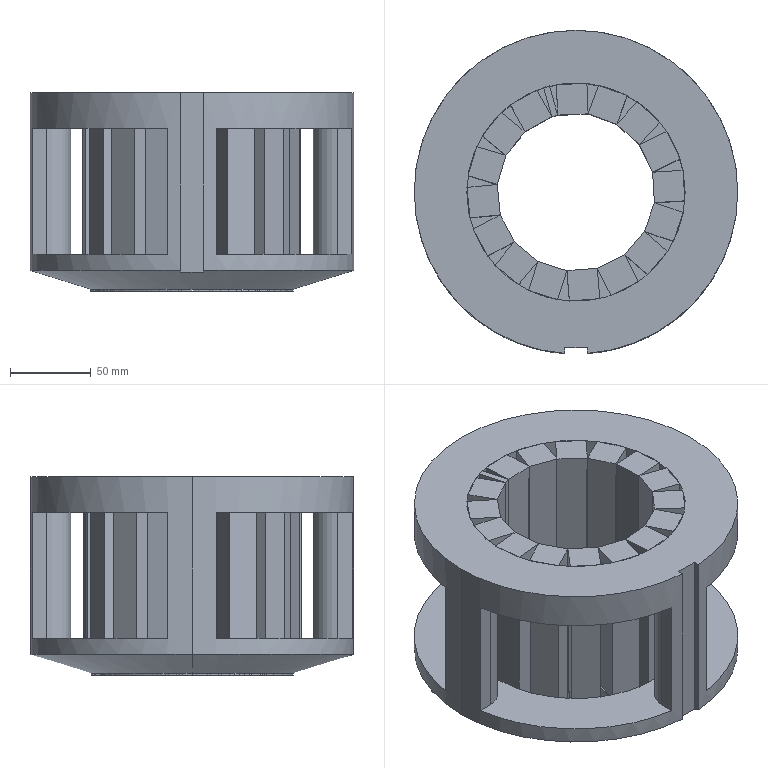Part | SolidWorks | features BaseBody 18 | 18 solids | 878 faces | box 200 x 199.755 x 123 mm | volume 1515679 mm3 | plane 857 | cylinder 17 | cone 4 | commonest cylinder face diameters 30 x8 135 x4 200 x3 125 x2